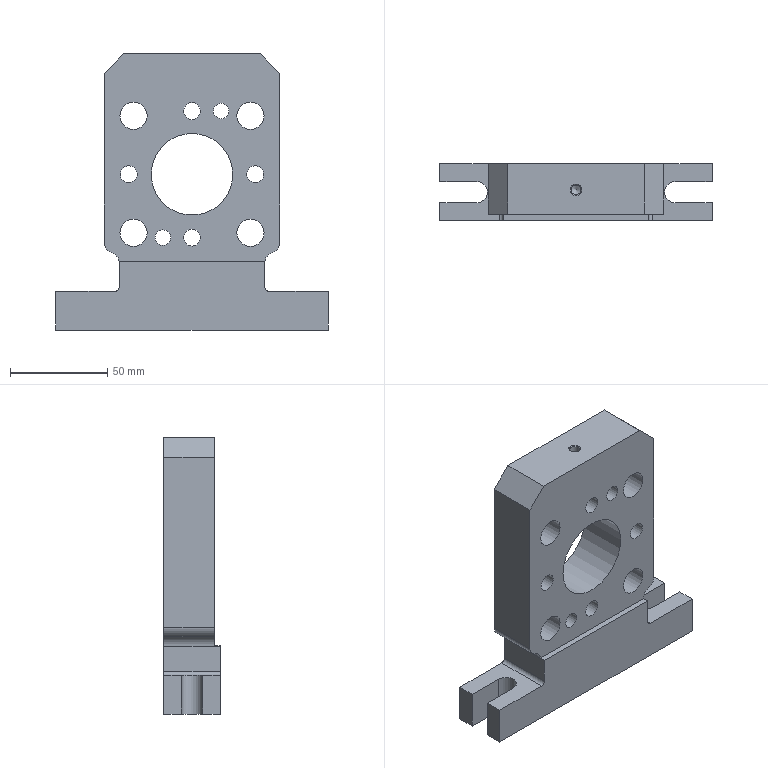Part | STEP file | 冲床-300配套压波_id942_x_t | 1 solid | 64 faces | box 140 x 29 x 142 mm | volume 284024 mm3 | cylinder 28 | plane 26 | cone 10 | commonest cylinder face diameters 14 x8 4.2 x4 8.7 x4 10 x4 4 x2 8 x2